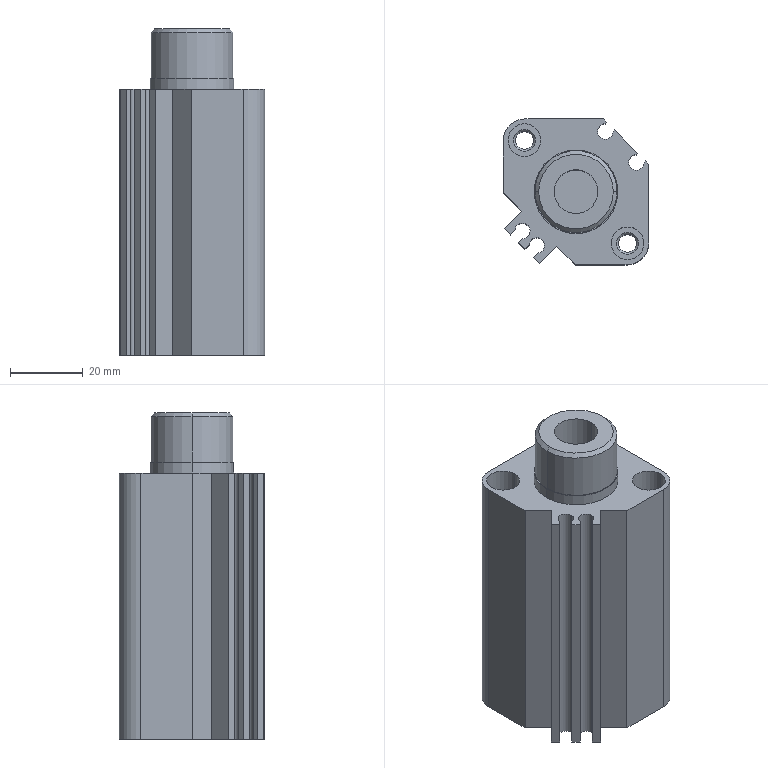Part | SolidWorks | features RefAxis 9, RevCut 5, 3DProfileFeature 3, Extrusion 1, Revolution 1 | 1 solid | 98 faces | box 40 x 40 x 89.5 mm | volume 78652 mm3 | cylinder 44 | plane 36 | cone 18 | commonest cylinder face diameters 4.25 x10 4.917 x8 9 x8 4.134 x4 5.5 x4 12 x4